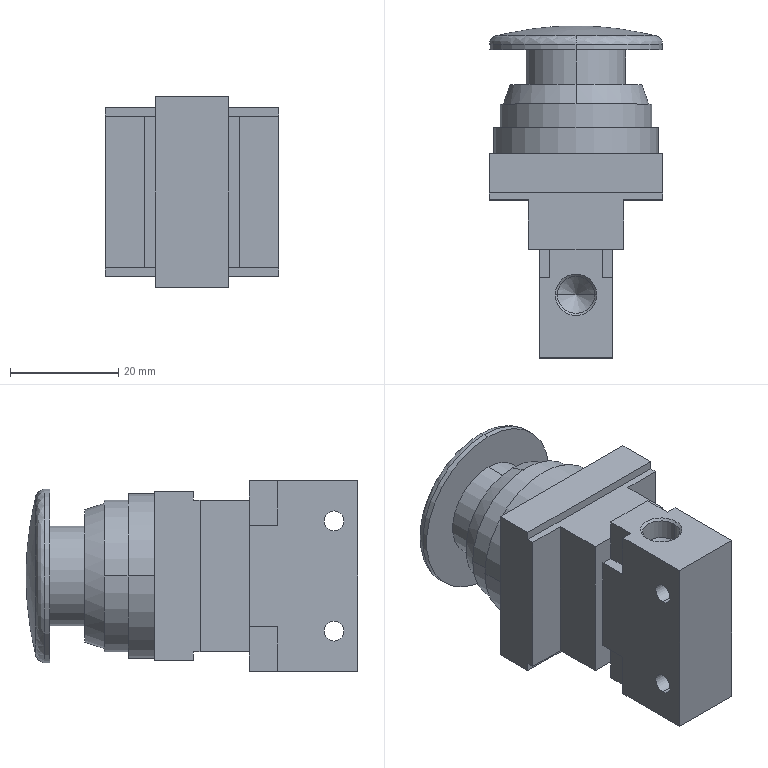Part | SolidWorks | features BaseBody 1 | 1 solid | 67 faces | box 32 x 61.2 x 35.2 mm | volume 33784 mm3 | plane 38 | cylinder 16 | cone 10 | spline 3 | commonest cylinder face diameters 3.68 x4 6.856 x4 18.4 x2 28 x2 30.4 x2 32 x2